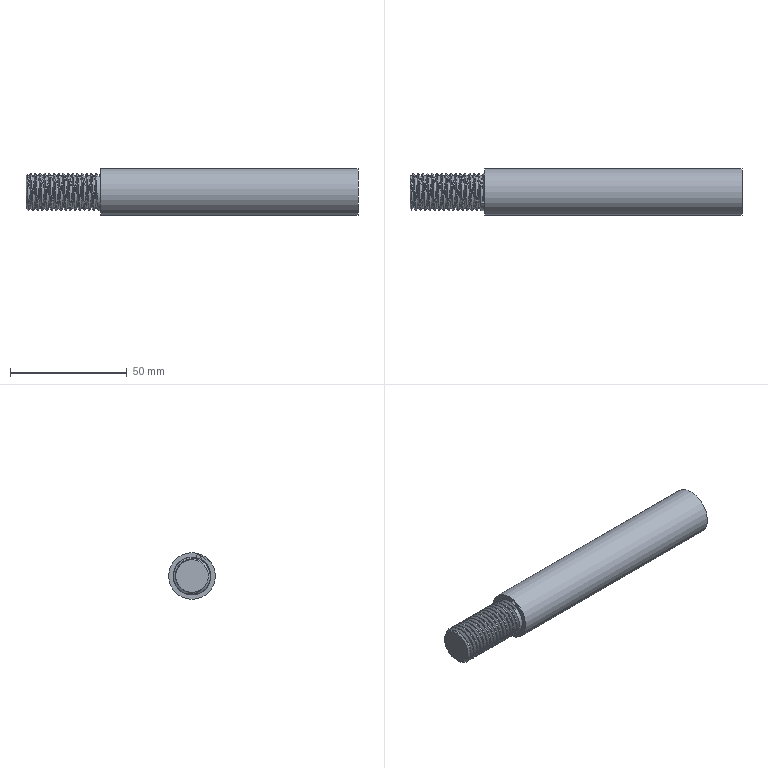Part | STEP file | Tube feed_id546_x_t | 1 solid | 11 faces | box 142 x 20 x 20 mm | volume 39874 mm3 | plane 4 | cylinder 3 | spline 3 | cone 1 | commonest cylinder face diameters 14 x1 16 x1 20 x1